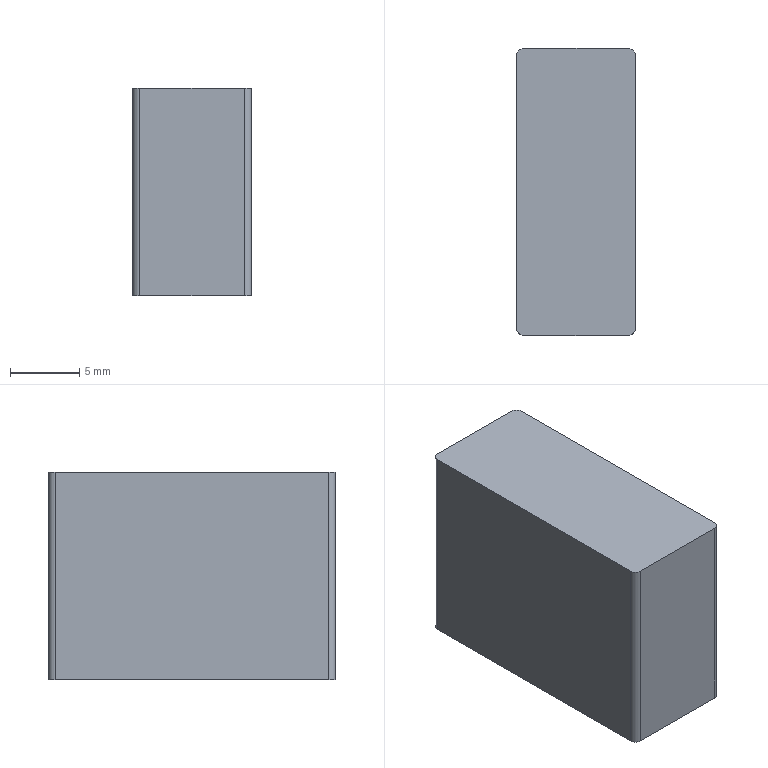Part | NX | features BREP 1 | 1 solid | 10 faces | box 8.558 x 20.702 x 15 mm | volume 2654 mm3 | plane 6 | cylinder 4 | commonest cylinder face diameters 1 x4
STEP:
#1=CARTESIAN_POINT('',(-3.779,10.351,-25.6));
#2=VERTEX_POINT('',#1);
#3=CARTESIAN_POINT('',(-4.279,9.851,-25.6));
#4=VERTEX_POINT('',#3);
#5=CARTESIAN_POINT('',(-3.779,9.851,-25.6));
#6=DIRECTION('',(0.,0.,1.));
#7=DIRECTION('',(1.,0.,0.));
#8=AXIS2_PLACEMENT_3D('',#5,#6,#7);
#9=CIRCLE('',#8,0.5);
#10=EDGE_CURVE('',#2,#4,#9,.T.);
#11=ORIENTED_EDGE('',*,*,#10,.F.);
#12=CARTESIAN_POINT('',(-3.779,10.351,-40.6));
#13=VERTEX_POINT('',#12);
#14=CARTESIAN_POINT('',(-3.779,10.351,-40.6));
#15=DIRECTION('',(0.,0.,1.));
#16=VECTOR('',#15,1000.);
#17=LINE('',#14,#16);
#18=EDGE_CURVE('',#13,#2,#17,.T.);
#19=ORIENTED_EDGE('',*,*,#18,.F.);
#20=CARTESIAN_POINT('',(-4.279,9.851,-40.6));
#21=VERTEX_POINT('',#20);
#22=CARTESIAN_POINT('',(-3.779,9.851,-40.6));
#23=DIRECTION('',(0.,0.,1.));
#24=DIRECTION('',(1.,0.,0.));
#25=AXIS2_PLACEMENT_3D('',#22,#23,#24);
#26=CIRCLE('',#25,0.5);
#27=EDGE_CURVE('',#13,#21,#26,.T.);
#28=ORIENTED_EDGE('',*,*,#27,.T.);
#29=CARTESIAN_POINT('',(-4.279,9.851,-40.6));
#30=DIRECTION('',(0.,0.,1.));
#31=VECTOR('',#30,1000.);
#32=LINE('',#29,#31);
#33=EDGE_CURVE('',#21,#4,#32,.T.);
#34=ORIENTED_EDGE('',*,*,#33,.T.);
#35=EDGE_LOOP('',(#11,#19,#28,#34));
#36=FACE_BOUND('',#35,.T.);
#37=CARTESIAN_POINT('',(-3.779,9.851,-40.6));
#38=DIRECTION('',(0.,0.,1.));
#39=DIRECTION('',(-1.,0.,0.));
#40=AXIS2_PLACEMENT_3D('',#37,#38,#39);
#41=CYLINDRICAL_SURFACE('',#40,0.5);
#42=ADVANCED_FACE('',(#36),#41,.T.);
#43=CARTESIAN_POINT('',(-4.279,-9.851,-25.6));
#44=VERTEX_POINT('',#43);
#45=CARTESIAN_POINT('',(-4.279,-9.851,-25.6));
#46=DIRECTION('',(0.,1.,0.));
#47=VECTOR('',#46,1000.);
#48=LINE('',#45,#47);
#49=EDGE_CURVE('',#44,#4,#48,.T.);
#50=ORIENTED_EDGE('',*,*,#49,.T.);
#51=ORIENTED_EDGE('',*,*,#33,.F.);
#52=CARTESIAN_POINT('',(-4.279,-9.851,-40.6));
#53=VERTEX_POINT('',#52);
#54=CARTESIAN_POINT('',(-4.279,-9.851,-40.6));
#55=DIRECTION('',(0.,1.,0.));
#56=VECTOR('',#55,1000.);
#57=LINE('',#54,#56);
#58=EDGE_CURVE('',#53,#21,#57,.T.);
#59=ORIENTED_EDGE('',*,*,#58,.F.);
#60=CARTESIAN_POINT('',(-4.279,-9.851,-40.6));
#61=DIRECTION('',(0.,0.,1.));
#62=VECTOR('',#61,1000.);
#63=LINE('',#60,#62);
#64=EDGE_CURVE('',#53,#44,#63,.T.);
#65=ORIENTED_EDGE('',*,*,#64,.T.);
#66=EDGE_LOOP('',(#50,#51,#59,#65));
#67=FACE_BOUND('',#66,.T.);
#68=CARTESIAN_POINT('',(-4.279,-9.851,-40.6));
#69=DIRECTION('',(1.,0.,0.));
#70=DIRECTION('',(0.,0.,1.));
#71=AXIS2_PLACEMENT_3D('',#68,#69,#70);
#72=PLANE('',#71);
#73=ADVANCED_FACE('',(#67),#72,.F.);
#74=CARTESIAN_POINT('',(-3.779,-10.351,-25.6));
#75=VERTEX_POINT('',#74);
#76=CARTESIAN_POINT('',(-3.779,-9.851,-25.6));
#77=DIRECTION('',(0.,0.,1.));
#78=DIRECTION('',(1.,0.,0.));
#79=AXIS2_PLACEMENT_3D('',#76,#77,#78);
#80=CIRCLE('',#79,0.5);
#81=EDGE_CURVE('',#44,#75,#80,.T.);
#82=ORIENTED_EDGE('',*,*,#81,.F.);
#83=ORIENTED_EDGE('',*,*,#64,.F.);
#84=CARTESIAN_POINT('',(-3.779,-10.351,-40.6));
#85=VERTEX_POINT('',#84);
#86=CARTESIAN_POINT('',(-3.779,-9.851,-40.6));
#87=DIRECTION('',(0.,0.,1.));
#88=DIRECTION('',(1.,0.,0.));
#89=AXIS2_PLACEMENT_3D('',#86,#87,#88);
#90=CIRCLE('',#89,0.5);
#91=EDGE_CURVE('',#53,#85,#90,.T.);
#92=ORIENTED_EDGE('',*,*,#91,.T.);
#93=CARTESIAN_POINT('',(-3.779,-10.351,-40.6));
#94=DIRECTION('',(0.,0.,1.));
#95=VECTOR('',#94,1000.);
#96=LINE('',#93,#95);
#97=EDGE_CURVE('',#85,#75,#96,.T.);
#98=ORIENTED_EDGE('',*,*,#97,.T.);
#99=EDGE_LOOP('',(#82,#83,#92,#98));
#100=FACE_BOUND('',#99,.T.);
#101=CARTESIAN_POINT('',(-3.779,-9.851,-40.6));
#102=DIRECTION('',(0.,0.,1.));
#103=DIRECTION('',(-1.,0.,0.));
#104=AXIS2_PLACEMENT_3D('',#101,#102,#103);
#105=CYLINDRICAL_SURFACE('',#104,0.5);
#106=ADVANCED_FACE('',(#100),#105,.T.);
#107=CARTESIAN_POINT('',(3.779,-10.351,-25.6));
#108=VERTEX_POINT('',#107);
#109=CARTESIAN_POINT('',(3.779,-10.351,-25.6));
#110=DIRECTION('',(-1.,0.,0.));
#111=VECTOR('',#110,1000.);
#112=LINE('',#109,#111);
#113=EDGE_CURVE('',#108,#75,#112,.T.);
#114=ORIENTED_EDGE('',*,*,#113,.T.);
#115=ORIENTED_EDGE('',*,*,#97,.F.);
#116=CARTESIAN_POINT('',(3.779,-10.351,-40.6));
#117=VERTEX_POINT('',#116);
#118=CARTESIAN_POINT('',(3.779,-10.351,-40.6));
#119=DIRECTION('',(-1.,0.,0.));
#120=VECTOR('',#119,1000.);
#121=LINE('',#118,#120);
#122=EDGE_CURVE('',#117,#85,#121,.T.);
#123=ORIENTED_EDGE('',*,*,#122,.F.);
#124=CARTESIAN_POINT('',(3.779,-10.351,-40.6));
#125=DIRECTION('',(0.,0.,1.));
#126=VECTOR('',#125,1000.);
#127=LINE('',#124,#126);
#128=EDGE_CURVE('',#117,#108,#127,.T.);
#129=ORIENTED_EDGE('',*,*,#128,.T.);
#130=EDGE_LOOP('',(#114,#115,#123,#129));
#131=FACE_BOUND('',#130,.T.);
#132=CARTESIAN_POINT('',(3.779,-10.351,-40.6));
#133=DIRECTION('',(0.,1.,0.));
#134=DIRECTION('',(0.,0.,-1.));
#135=AXIS2_PLACEMENT_3D('',#132,#133,#134);
#136=PLANE('',#135);
#137=ADVANCED_FACE('',(#131),#136,.F.);
#138=CARTESIAN_POINT('',(4.279,-9.851,-25.6));
#139=VERTEX_POINT('',#138);
#140=CARTESIAN_POINT('',(3.779,-9.851,-25.6));
#141=DIRECTION('',(0.,0.,1.));
#142=DIRECTION('',(1.,0.,0.));
#143=AXIS2_PLACEMENT_3D('',#140,#141,#142);
#144=CIRCLE('',#143,0.5);
#145=EDGE_CURVE('',#108,#139,#144,.T.);
#146=ORIENTED_EDGE('',*,*,#145,.F.);
#147=ORIENTED_EDGE('',*,*,#128,.F.);
#148=CARTESIAN_POINT('',(4.279,-9.851,-40.6));
#149=VERTEX_POINT('',#148);
#150=CARTESIAN_POINT('',(3.779,-9.851,-40.6));
#151=DIRECTION('',(0.,0.,1.));
#152=DIRECTION('',(1.,0.,0.));
#153=AXIS2_PLACEMENT_3D('',#150,#151,#152);
#154=CIRCLE('',#153,0.5);
#155=EDGE_CURVE('',#117,#149,#154,.T.);
#156=ORIENTED_EDGE('',*,*,#155,.T.);
#157=CARTESIAN_POINT('',(4.279,-9.851,-40.6));
#158=DIRECTION('',(0.,0.,1.));
#159=VECTOR('',#158,1000.);
#160=LINE('',#157,#159);
#161=EDGE_CURVE('',#149,#139,#160,.T.);
#162=ORIENTED_EDGE('',*,*,#161,.T.);
#163=EDGE_LOOP('',(#146,#147,#156,#162));
#164=FACE_BOUND('',#163,.T.);
#165=CARTESIAN_POINT('',(3.779,-9.851,-40.6));
#166=DIRECTION('',(0.,0.,1.));
#167=DIRECTION('',(-1.,0.,0.));
#168=AXIS2_PLACEMENT_3D('',#165,#166,#167);
#169=CYLINDRICAL_SURFACE('',#168,0.5);
#170=ADVANCED_FACE('',(#164),#169,.T.);
#171=CARTESIAN_POINT('',(4.279,9.851,-25.6));
#172=VERTEX_POINT('',#171);
#173=CARTESIAN_POINT('',(4.279,9.851,-25.6));
#174=DIRECTION('',(0.,-1.,0.));
#175=VECTOR('',#174,1000.);
#176=LINE('',#173,#175);
#177=EDGE_CURVE('',#172,#139,#176,.T.);
#178=ORIENTED_EDGE('',*,*,#177,.T.);
#179=ORIENTED_EDGE('',*,*,#161,.F.);
#180=CARTESIAN_POINT('',(4.279,9.851,-40.6));
#181=VERTEX_POINT('',#180);
#182=CARTESIAN_POINT('',(4.279,9.851,-40.6));
#183=DIRECTION('',(0.,-1.,0.));
#184=VECTOR('',#183,1000.);
#185=LINE('',#182,#184);
#186=EDGE_CURVE('',#181,#149,#185,.T.);
#187=ORIENTED_EDGE('',*,*,#186,.F.);
#188=CARTESIAN_POINT('',(4.279,9.851,-40.6));
#189=DIRECTION('',(0.,0.,1.));
#190=VECTOR('',#189,1000.);
#191=LINE('',#188,#190);
#192=EDGE_CURVE('',#181,#172,#191,.T.);
#193=ORIENTED_EDGE('',*,*,#192,.T.);
#194=EDGE_LOOP('',(#178,#179,#187,#193));
#195=FACE_BOUND('',#194,.T.);
#196=CARTESIAN_POINT('',(4.279,9.851,-40.6));
#197=DIRECTION('',(-1.,0.,0.));
#198=DIRECTION('',(0.,1.,0.));
#199=AXIS2_PLACEMENT_3D('',#196,#197,#198);
#200=PLANE('',#199);
#201=ADVANCED_FACE('',(#195),#200,.F.);
#202=CARTESIAN_POINT('',(3.779,10.351,-25.6));
#203=VERTEX_POINT('',#202);
#204=CARTESIAN_POINT('',(3.779,9.851,-25.6));
#205=DIRECTION('',(0.,0.,1.));
#206=DIRECTION('',(1.,0.,0.));
#207=AXIS2_PLACEMENT_3D('',#204,#205,#206);
#208=CIRCLE('',#207,0.5);
#209=EDGE_CURVE('',#172,#203,#208,.T.);
#210=ORIENTED_EDGE('',*,*,#209,.F.);
#211=ORIENTED_EDGE('',*,*,#192,.F.);
#212=CARTESIAN_POINT('',(3.779,10.351,-40.6));
#213=VERTEX_POINT('',#212);
#214=CARTESIAN_POINT('',(3.779,9.851,-40.6));
#215=DIRECTION('',(0.,0.,1.));
#216=DIRECTION('',(1.,0.,0.));
#217=AXIS2_PLACEMENT_3D('',#214,#215,#216);
#218=CIRCLE('',#217,0.5);
#219=EDGE_CURVE('',#181,#213,#218,.T.);
#220=ORIENTED_EDGE('',*,*,#219,.T.);
#221=CARTESIAN_POINT('',(3.779,10.351,-40.6));
#222=DIRECTION('',(0.,0.,1.));
#223=VECTOR('',#222,1000.);
#224=LINE('',#221,#223);
#225=EDGE_CURVE('',#213,#203,#224,.T.);
#226=ORIENTED_EDGE('',*,*,#225,.T.);
#227=EDGE_LOOP('',(#210,#211,#220,#226));
#228=FACE_BOUND('',#227,.T.);
#229=CARTESIAN_POINT('',(3.779,9.851,-40.6));
#230=DIRECTION('',(0.,0.,1.));
#231=DIRECTION('',(-1.,0.,0.));
#232=AXIS2_PLACEMENT_3D('',#229,#230,#231);
#233=CYLINDRICAL_SURFACE('',#232,0.5);
#234=ADVANCED_FACE('',(#228),#233,.T.);
#235=CARTESIAN_POINT('',(-3.779,10.351,-25.6));
#236=DIRECTION('',(1.,0.,0.));
#237=VECTOR('',#236,1000.);
#238=LINE('',#235,#237);
#239=EDGE_CURVE('',#2,#203,#238,.T.);
#240=ORIENTED_EDGE('',*,*,#239,.T.);
#241=ORIENTED_EDGE('',*,*,#225,.F.);
#242=CARTESIAN_POINT('',(-3.779,10.351,-40.6));
#243=DIRECTION('',(1.,0.,0.));
#244=VECTOR('',#243,1000.);
#245=LINE('',#242,#244);
#246=EDGE_CURVE('',#13,#213,#245,.T.);
#247=ORIENTED_EDGE('',*,*,#246,.F.);
#248=ORIENTED_EDGE('',*,*,#18,.T.);
#249=EDGE_LOOP('',(#240,#241,#247,#248));
#250=FACE_BOUND('',#249,.T.);
#251=CARTESIAN_POINT('',(-3.779,10.351,-40.6));
#252=DIRECTION('',(0.,-1.,0.));
#253=DIRECTION('',(0.,0.,1.));
#254=AXIS2_PLACEMENT_3D('',#251,#252,#253);
#255=PLANE('',#254);
#256=ADVANCED_FACE('',(#250),#255,.F.);
#257=ORIENTED_EDGE('',*,*,#27,.F.);
#258=ORIENTED_EDGE('',*,*,#246,.T.);
#259=ORIENTED_EDGE('',*,*,#219,.F.);
#260=ORIENTED_EDGE('',*,*,#186,.T.);
#261=ORIENTED_EDGE('',*,*,#155,.F.);
#262=ORIENTED_EDGE('',*,*,#122,.T.);
#263=ORIENTED_EDGE('',*,*,#91,.F.);
#264=ORIENTED_EDGE('',*,*,#58,.T.);
#265=EDGE_LOOP('',(#257,#258,#259,#260,#261,#262,#263,#264));
#266=FACE_BOUND('',#265,.T.);
#267=CARTESIAN_POINT('',(-3.779,9.851,-40.6));
#268=DIRECTION('',(0.,0.,1.));
#269=DIRECTION('',(-1.,0.,0.));
#270=AXIS2_PLACEMENT_3D('',#267,#268,#269);
#271=PLANE('',#270);
#272=ADVANCED_FACE('',(#266),#271,.F.);
#273=ORIENTED_EDGE('',*,*,#10,.T.);
#274=ORIENTED_EDGE('',*,*,#49,.F.);
#275=ORIENTED_EDGE('',*,*,#81,.T.);
#276=ORIENTED_EDGE('',*,*,#113,.F.);
#277=ORIENTED_EDGE('',*,*,#145,.T.);
#278=ORIENTED_EDGE('',*,*,#177,.F.);
#279=ORIENTED_EDGE('',*,*,#209,.T.);
#280=ORIENTED_EDGE('',*,*,#239,.F.);
#281=EDGE_LOOP('',(#273,#274,#275,#276,#277,#278,#279,#280));
#282=FACE_BOUND('',#281,.T.);
#283=CARTESIAN_POINT('',(-3.779,9.851,-25.6));
#284=DIRECTION('',(0.,0.,1.));
#285=DIRECTION('',(-1.,0.,0.));
#286=AXIS2_PLACEMENT_3D('',#283,#284,#285);
#287=PLANE('',#286);
#288=ADVANCED_FACE('',(#282),#287,.T.);
#289=CLOSED_SHELL('',(#42,#73,#106,#137,#170,#201,#234,#256,#272,#288));
#290=MANIFOLD_SOLID_BREP('',#289);
#291=(LENGTH_UNIT()NAMED_UNIT(*)SI_UNIT(.MILLI.,.METRE.));
#292=UNCERTAINTY_MEASURE_WITH_UNIT(LENGTH_MEASURE(0.00001),#291,'','');
#293=(NAMED_UNIT(*)PLANE_ANGLE_UNIT()SI_UNIT($,.RADIAN.));
#294=(NAMED_UNIT(*)SI_UNIT($,.STERADIAN.)SOLID_ANGLE_UNIT());
#295=(GEOMETRIC_REPRESENTATION_CONTEXT(3)GLOBAL_UNCERTAINTY_ASSIGNED_CONTEXT((#292))GLOBAL_UNIT_ASSIGNED_CONTEXT((#291,#293,#294))REPRESENTATION_CONTEXT('',''));
#296=ADVANCED_BREP_SHAPE_REPRESENTATION('',(#290),#295);